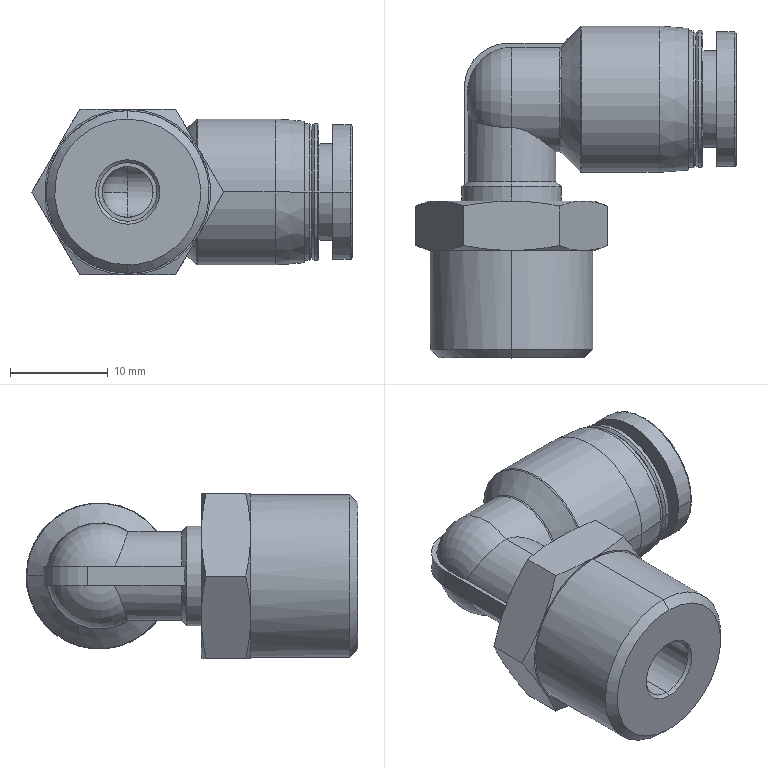Part | SolidWorks | features BaseBody 1 | 1 solid | 89 faces | box 32.815 x 34 x 17 mm | volume 6015 mm3 | cone 28 | cylinder 27 | plane 19 | torus 13 | sphere 2 | commonest cylinder face diameters 5.2 x4 14 x4 9.08 x3 6 x2 8 x2 9.9 x2